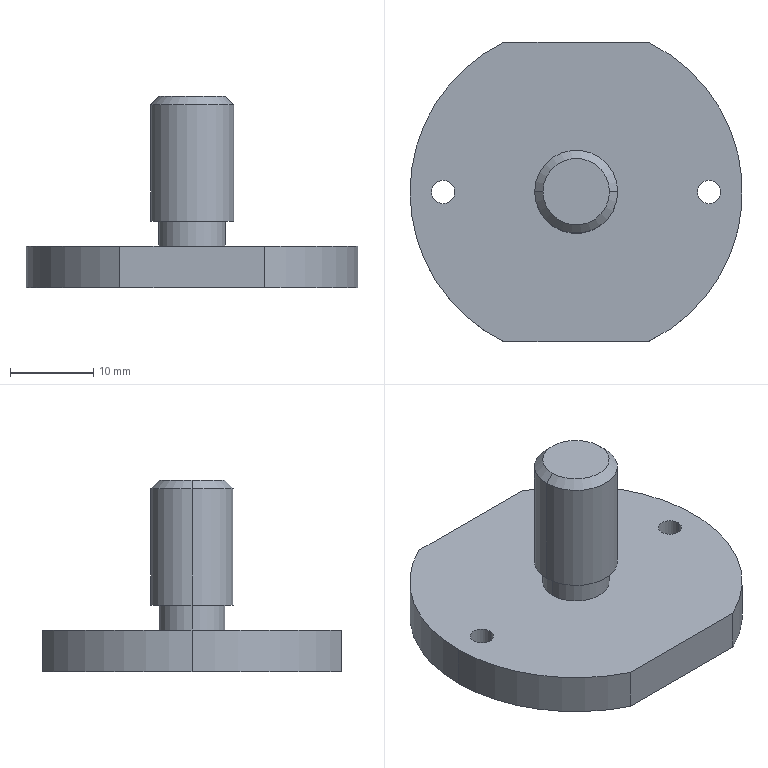Part | STEP file | Motor pulley screw | 1 solid | 19 faces | box 40 x 36 x 23 mm | volume 7301 mm3 | cylinder 11 | plane 6 | cone 2 | commonest cylinder face diameters 2.8 x4 40 x3 8 x2 10 x2
STEP:
#1=CARTESIAN_POINT('',(-14.6,0.,0.));
#2=VERTEX_POINT('',#1);
#3=CARTESIAN_POINT('',(-17.4,0.,0.));
#4=VERTEX_POINT('',#3);
#5=CARTESIAN_POINT('',(-16.,0.,0.));
#6=DIRECTION('',(0.,0.,-1.));
#7=DIRECTION('',(1.,0.,0.));
#8=AXIS2_PLACEMENT_3D('',#5,#6,#7);
#9=CIRCLE('',#8,1.4);
#10=EDGE_CURVE('',#2,#4,#9,.T.);
#11=ORIENTED_EDGE('',*,*,#10,.T.);
#12=CARTESIAN_POINT('',(-17.4,0.,5.));
#13=VERTEX_POINT('',#12);
#14=CARTESIAN_POINT('',(-17.4,0.,-10.));
#15=DIRECTION('',(0.,0.,1.));
#16=VECTOR('',#15,1000.);
#17=LINE('',#14,#16);
#18=EDGE_CURVE('',#4,#13,#17,.T.);
#19=ORIENTED_EDGE('',*,*,#18,.T.);
#20=CARTESIAN_POINT('',(-14.6,0.,5.));
#21=VERTEX_POINT('',#20);
#22=CARTESIAN_POINT('',(-16.,0.,5.));
#23=DIRECTION('',(0.,0.,-1.));
#24=DIRECTION('',(-1.,0.,0.));
#25=AXIS2_PLACEMENT_3D('',#22,#23,#24);
#26=CIRCLE('',#25,1.4);
#27=EDGE_CURVE('',#21,#13,#26,.T.);
#28=ORIENTED_EDGE('',*,*,#27,.F.);
#29=CARTESIAN_POINT('',(-14.6,0.,-10.));
#30=DIRECTION('',(0.,0.,1.));
#31=VECTOR('',#30,1000.);
#32=LINE('',#29,#31);
#33=EDGE_CURVE('',#2,#21,#32,.T.);
#34=ORIENTED_EDGE('',*,*,#33,.F.);
#35=EDGE_LOOP('',(#11,#19,#28,#34));
#36=FACE_OUTER_BOUND('',#35,.T.);
#37=CARTESIAN_POINT('',(-16.,0.,-10.));
#38=DIRECTION('',(0.,0.,1.));
#39=DIRECTION('',(1.,0.,0.));
#40=AXIS2_PLACEMENT_3D('',#37,#38,#39);
#41=CYLINDRICAL_SURFACE('',#40,1.4);
#42=ADVANCED_FACE('',(#36),#41,.F.);
#43=CARTESIAN_POINT('',(14.6,0.,0.));
#44=VERTEX_POINT('',#43);
#45=CARTESIAN_POINT('',(17.4,0.,0.));
#46=VERTEX_POINT('',#45);
#47=CARTESIAN_POINT('',(16.,0.,0.));
#48=DIRECTION('',(0.,0.,1.));
#49=DIRECTION('',(1.,0.,0.));
#50=AXIS2_PLACEMENT_3D('',#47,#48,#49);
#51=CIRCLE('',#50,1.4);
#52=EDGE_CURVE('',#44,#46,#51,.T.);
#53=ORIENTED_EDGE('',*,*,#52,.F.);
#54=CARTESIAN_POINT('',(14.6,0.,5.));
#55=VERTEX_POINT('',#54);
#56=CARTESIAN_POINT('',(14.6,0.,-10.));
#57=DIRECTION('',(0.,0.,1.));
#58=VECTOR('',#57,1000.);
#59=LINE('',#56,#58);
#60=EDGE_CURVE('',#44,#55,#59,.T.);
#61=ORIENTED_EDGE('',*,*,#60,.T.);
#62=CARTESIAN_POINT('',(17.4,0.,5.));
#63=VERTEX_POINT('',#62);
#64=CARTESIAN_POINT('',(16.,0.,5.));
#65=DIRECTION('',(0.,0.,1.));
#66=DIRECTION('',(1.,0.,0.));
#67=AXIS2_PLACEMENT_3D('',#64,#65,#66);
#68=CIRCLE('',#67,1.4);
#69=EDGE_CURVE('',#55,#63,#68,.T.);
#70=ORIENTED_EDGE('',*,*,#69,.T.);
#71=CARTESIAN_POINT('',(17.4,0.,-10.));
#72=DIRECTION('',(0.,0.,1.));
#73=VECTOR('',#72,1000.);
#74=LINE('',#71,#73);
#75=EDGE_CURVE('',#46,#63,#74,.T.);
#76=ORIENTED_EDGE('',*,*,#75,.F.);
#77=EDGE_LOOP('',(#53,#61,#70,#76));
#78=FACE_OUTER_BOUND('',#77,.T.);
#79=CARTESIAN_POINT('',(16.,0.,-10.));
#80=DIRECTION('',(0.,0.,1.));
#81=DIRECTION('',(1.,0.,0.));
#82=AXIS2_PLACEMENT_3D('',#79,#80,#81);
#83=CYLINDRICAL_SURFACE('',#82,1.4);
#84=ADVANCED_FACE('',(#78),#83,.F.);
#85=CARTESIAN_POINT('',(4.,0.,23.));
#86=VERTEX_POINT('',#85);
#87=CARTESIAN_POINT('',(-4.,0.,23.));
#88=VERTEX_POINT('',#87);
#89=CARTESIAN_POINT('',(0.,0.,23.));
#90=DIRECTION('',(0.,0.,1.));
#91=DIRECTION('',(1.,0.,0.));
#92=AXIS2_PLACEMENT_3D('',#89,#90,#91);
#93=CIRCLE('',#92,4.);
#94=EDGE_CURVE('',#86,#88,#93,.T.);
#95=ORIENTED_EDGE('',*,*,#94,.F.);
#96=CARTESIAN_POINT('',(5.,0.,22.));
#97=VERTEX_POINT('',#96);
#98=CARTESIAN_POINT('',(4.,0.,23.));
#99=DIRECTION('',(0.7071,0.,-0.7071));
#100=VECTOR('',#99,1000.);
#101=LINE('',#98,#100);
#102=EDGE_CURVE('',#86,#97,#101,.T.);
#103=ORIENTED_EDGE('',*,*,#102,.T.);
#104=CARTESIAN_POINT('',(-5.,0.,22.));
#105=VERTEX_POINT('',#104);
#106=CARTESIAN_POINT('',(0.,0.,22.));
#107=DIRECTION('',(0.,0.,-1.));
#108=DIRECTION('',(1.,0.,0.));
#109=AXIS2_PLACEMENT_3D('',#106,#107,#108);
#110=CIRCLE('',#109,5.);
#111=EDGE_CURVE('',#105,#97,#110,.T.);
#112=ORIENTED_EDGE('',*,*,#111,.F.);
#113=CARTESIAN_POINT('',(-4.,0.,23.));
#114=DIRECTION('',(-0.7071,0.,-0.7071));
#115=VECTOR('',#114,1000.);
#116=LINE('',#113,#115);
#117=EDGE_CURVE('',#88,#105,#116,.T.);
#118=ORIENTED_EDGE('',*,*,#117,.F.);
#119=EDGE_LOOP('',(#95,#103,#112,#118));
#120=FACE_OUTER_BOUND('',#119,.T.);
#121=CARTESIAN_POINT('',(0.,0.,23.));
#122=DIRECTION('',(0.,0.,-1.));
#123=DIRECTION('',(-1.,0.,0.));
#124=AXIS2_PLACEMENT_3D('',#121,#122,#123);
#125=CONICAL_SURFACE('',#124,4.,0.7854);
#126=ADVANCED_FACE('',(#120),#125,.T.);
#127=ORIENTED_EDGE('',*,*,#111,.T.);
#128=CARTESIAN_POINT('',(5.,0.,8.));
#129=VERTEX_POINT('',#128);
#130=CARTESIAN_POINT('',(5.,0.,23.));
#131=DIRECTION('',(0.,0.,-1.));
#132=VECTOR('',#131,1000.);
#133=LINE('',#130,#132);
#134=EDGE_CURVE('',#97,#129,#133,.T.);
#135=ORIENTED_EDGE('',*,*,#134,.T.);
#136=CARTESIAN_POINT('',(-5.,0.,8.));
#137=VERTEX_POINT('',#136);
#138=CARTESIAN_POINT('',(0.,0.,8.));
#139=DIRECTION('',(0.,0.,1.));
#140=DIRECTION('',(1.,0.,0.));
#141=AXIS2_PLACEMENT_3D('',#138,#139,#140);
#142=CIRCLE('',#141,5.);
#143=EDGE_CURVE('',#129,#137,#142,.T.);
#144=ORIENTED_EDGE('',*,*,#143,.T.);
#145=CARTESIAN_POINT('',(-5.,0.,23.));
#146=DIRECTION('',(0.,0.,-1.));
#147=VECTOR('',#146,1000.);
#148=LINE('',#145,#147);
#149=EDGE_CURVE('',#105,#137,#148,.T.);
#150=ORIENTED_EDGE('',*,*,#149,.F.);
#151=EDGE_LOOP('',(#127,#135,#144,#150));
#152=FACE_OUTER_BOUND('',#151,.T.);
#153=CARTESIAN_POINT('',(0.,0.,23.));
#154=DIRECTION('',(0.,0.,-1.));
#155=DIRECTION('',(-1.,0.,0.));
#156=AXIS2_PLACEMENT_3D('',#153,#154,#155);
#157=CYLINDRICAL_SURFACE('',#156,5.);
#158=ADVANCED_FACE('',(#152),#157,.T.);
#159=CARTESIAN_POINT('',(4.,0.,8.));
#160=VERTEX_POINT('',#159);
#161=CARTESIAN_POINT('',(-4.,0.,8.));
#162=VERTEX_POINT('',#161);
#163=CARTESIAN_POINT('',(0.,0.,8.));
#164=DIRECTION('',(0.,0.,1.));
#165=DIRECTION('',(1.,0.,0.));
#166=AXIS2_PLACEMENT_3D('',#163,#164,#165);
#167=CIRCLE('',#166,4.);
#168=EDGE_CURVE('',#160,#162,#167,.T.);
#169=ORIENTED_EDGE('',*,*,#168,.F.);
#170=CARTESIAN_POINT('',(4.,0.,5.));
#171=VERTEX_POINT('',#170);
#172=CARTESIAN_POINT('',(4.,0.,8.));
#173=DIRECTION('',(0.,0.,-1.));
#174=VECTOR('',#173,1000.);
#175=LINE('',#172,#174);
#176=EDGE_CURVE('',#160,#171,#175,.T.);
#177=ORIENTED_EDGE('',*,*,#176,.T.);
#178=CARTESIAN_POINT('',(-4.,0.,5.));
#179=VERTEX_POINT('',#178);
#180=CARTESIAN_POINT('',(0.,0.,5.));
#181=DIRECTION('',(0.,0.,1.));
#182=DIRECTION('',(1.,0.,0.));
#183=AXIS2_PLACEMENT_3D('',#180,#181,#182);
#184=CIRCLE('',#183,4.);
#185=EDGE_CURVE('',#171,#179,#184,.T.);
#186=ORIENTED_EDGE('',*,*,#185,.T.);
#187=CARTESIAN_POINT('',(-4.,0.,8.));
#188=DIRECTION('',(0.,0.,-1.));
#189=VECTOR('',#188,1000.);
#190=LINE('',#187,#189);
#191=EDGE_CURVE('',#162,#179,#190,.T.);
#192=ORIENTED_EDGE('',*,*,#191,.F.);
#193=EDGE_LOOP('',(#169,#177,#186,#192));
#194=FACE_OUTER_BOUND('',#193,.T.);
#195=CARTESIAN_POINT('',(0.,0.,8.));
#196=DIRECTION('',(0.,0.,-1.));
#197=DIRECTION('',(-1.,0.,0.));
#198=AXIS2_PLACEMENT_3D('',#195,#196,#197);
#199=CYLINDRICAL_SURFACE('',#198,4.);
#200=ADVANCED_FACE('',(#194),#199,.T.);
#201=CARTESIAN_POINT('',(-20.,0.,5.));
#202=VERTEX_POINT('',#201);
#203=CARTESIAN_POINT('',(-8.718,-18.,5.));
#204=VERTEX_POINT('',#203);
#205=CARTESIAN_POINT('',(0.,0.,5.));
#206=DIRECTION('',(0.,0.,1.));
#207=DIRECTION('',(1.,0.,0.));
#208=AXIS2_PLACEMENT_3D('',#205,#206,#207);
#209=CIRCLE('',#208,20.);
#210=EDGE_CURVE('',#202,#204,#209,.T.);
#211=ORIENTED_EDGE('',*,*,#210,.F.);
#212=CARTESIAN_POINT('',(-20.,0.,0.));
#213=VERTEX_POINT('',#212);
#214=CARTESIAN_POINT('',(-20.,0.,5.));
#215=DIRECTION('',(0.,0.,-1.));
#216=VECTOR('',#215,1000.);
#217=LINE('',#214,#216);
#218=EDGE_CURVE('',#202,#213,#217,.T.);
#219=ORIENTED_EDGE('',*,*,#218,.T.);
#220=CARTESIAN_POINT('',(-8.718,-18.,0.));
#221=VERTEX_POINT('',#220);
#222=CARTESIAN_POINT('',(0.,0.,0.));
#223=DIRECTION('',(0.,0.,1.));
#224=DIRECTION('',(1.,0.,0.));
#225=AXIS2_PLACEMENT_3D('',#222,#223,#224);
#226=CIRCLE('',#225,20.);
#227=EDGE_CURVE('',#213,#221,#226,.T.);
#228=ORIENTED_EDGE('',*,*,#227,.T.);
#229=CARTESIAN_POINT('',(-8.718,-18.,5.));
#230=DIRECTION('',(0.,0.,-1.));
#231=VECTOR('',#230,1000.);
#232=LINE('',#229,#231);
#233=EDGE_CURVE('',#204,#221,#232,.T.);
#234=ORIENTED_EDGE('',*,*,#233,.F.);
#235=EDGE_LOOP('',(#211,#219,#228,#234));
#236=FACE_OUTER_BOUND('',#235,.T.);
#237=CARTESIAN_POINT('',(0.,0.,5.));
#238=DIRECTION('',(0.,0.,-1.));
#239=DIRECTION('',(-1.,0.,0.));
#240=AXIS2_PLACEMENT_3D('',#237,#238,#239);
#241=CYLINDRICAL_SURFACE('',#240,20.);
#242=ADVANCED_FACE('',(#236),#241,.T.);
#243=ORIENTED_EDGE('',*,*,#218,.F.);
#244=CARTESIAN_POINT('',(-8.718,18.,5.));
#245=VERTEX_POINT('',#244);
#246=CARTESIAN_POINT('',(0.,0.,5.));
#247=DIRECTION('',(0.,0.,1.));
#248=DIRECTION('',(1.,0.,0.));
#249=AXIS2_PLACEMENT_3D('',#246,#247,#248);
#250=CIRCLE('',#249,20.);
#251=EDGE_CURVE('',#245,#202,#250,.T.);
#252=ORIENTED_EDGE('',*,*,#251,.F.);
#253=CARTESIAN_POINT('',(-8.718,18.,0.));
#254=VERTEX_POINT('',#253);
#255=CARTESIAN_POINT('',(-8.718,18.,5.));
#256=DIRECTION('',(0.,0.,-1.));
#257=VECTOR('',#256,1000.);
#258=LINE('',#255,#257);
#259=EDGE_CURVE('',#245,#254,#258,.T.);
#260=ORIENTED_EDGE('',*,*,#259,.T.);
#261=CARTESIAN_POINT('',(0.,0.,0.));
#262=DIRECTION('',(0.,0.,1.));
#263=DIRECTION('',(1.,0.,0.));
#264=AXIS2_PLACEMENT_3D('',#261,#262,#263);
#265=CIRCLE('',#264,20.);
#266=EDGE_CURVE('',#254,#213,#265,.T.);
#267=ORIENTED_EDGE('',*,*,#266,.T.);
#268=EDGE_LOOP('',(#243,#252,#260,#267));
#269=FACE_OUTER_BOUND('',#268,.T.);
#270=CARTESIAN_POINT('',(0.,0.,5.));
#271=DIRECTION('',(0.,0.,-1.));
#272=DIRECTION('',(-1.,0.,0.));
#273=AXIS2_PLACEMENT_3D('',#270,#271,#272);
#274=CYLINDRICAL_SURFACE('',#273,20.);
#275=ADVANCED_FACE('',(#269),#274,.T.);
#276=CARTESIAN_POINT('',(8.718,-18.,0.));
#277=VERTEX_POINT('',#276);
#278=CARTESIAN_POINT('',(8.718,-18.,5.));
#279=VERTEX_POINT('',#278);
#280=CARTESIAN_POINT('',(8.718,-18.,5.));
#281=DIRECTION('',(0.,0.,1.));
#282=VECTOR('',#281,1000.);
#283=LINE('',#280,#282);
#284=EDGE_CURVE('',#277,#279,#283,.T.);
#285=ORIENTED_EDGE('',*,*,#284,.F.);
#286=CARTESIAN_POINT('',(8.718,18.,0.));
#287=VERTEX_POINT('',#286);
#288=CARTESIAN_POINT('',(0.,0.,0.));
#289=DIRECTION('',(0.,0.,1.));
#290=DIRECTION('',(1.,0.,0.));
#291=AXIS2_PLACEMENT_3D('',#288,#289,#290);
#292=CIRCLE('',#291,20.);
#293=EDGE_CURVE('',#277,#287,#292,.T.);
#294=ORIENTED_EDGE('',*,*,#293,.T.);
#295=CARTESIAN_POINT('',(8.718,18.,5.));
#296=VERTEX_POINT('',#295);
#297=CARTESIAN_POINT('',(8.718,18.,5.));
#298=DIRECTION('',(0.,0.,1.));
#299=VECTOR('',#298,1000.);
#300=LINE('',#297,#299);
#301=EDGE_CURVE('',#287,#296,#300,.T.);
#302=ORIENTED_EDGE('',*,*,#301,.T.);
#303=CARTESIAN_POINT('',(0.,0.,5.));
#304=DIRECTION('',(0.,0.,1.));
#305=DIRECTION('',(1.,0.,0.));
#306=AXIS2_PLACEMENT_3D('',#303,#304,#305);
#307=CIRCLE('',#306,20.);
#308=EDGE_CURVE('',#279,#296,#307,.T.);
#309=ORIENTED_EDGE('',*,*,#308,.F.);
#310=EDGE_LOOP('',(#285,#294,#302,#309));
#311=FACE_OUTER_BOUND('',#310,.T.);
#312=CARTESIAN_POINT('',(0.,0.,5.));
#313=DIRECTION('',(0.,0.,-1.));
#314=DIRECTION('',(-1.,0.,0.));
#315=AXIS2_PLACEMENT_3D('',#312,#313,#314);
#316=CYLINDRICAL_SURFACE('',#315,20.);
#317=ADVANCED_FACE('',(#311),#316,.T.);
#318=ORIENTED_EDGE('',*,*,#27,.T.);
#319=CARTESIAN_POINT('',(-16.,0.,5.));
#320=DIRECTION('',(0.,0.,-1.));
#321=DIRECTION('',(-1.,0.,0.));
#322=AXIS2_PLACEMENT_3D('',#319,#320,#321);
#323=CIRCLE('',#322,1.4);
#324=EDGE_CURVE('',#13,#21,#323,.T.);
#325=ORIENTED_EDGE('',*,*,#324,.T.);
#326=EDGE_LOOP('',(#318,#325));
#327=FACE_BOUND('',#326,.T.);
#328=CARTESIAN_POINT('',(16.,0.,5.));
#329=DIRECTION('',(0.,0.,1.));
#330=DIRECTION('',(1.,0.,0.));
#331=AXIS2_PLACEMENT_3D('',#328,#329,#330);
#332=CIRCLE('',#331,1.4);
#333=EDGE_CURVE('',#63,#55,#332,.T.);
#334=ORIENTED_EDGE('',*,*,#333,.F.);
#335=ORIENTED_EDGE('',*,*,#69,.F.);
#336=EDGE_LOOP('',(#334,#335));
#337=FACE_BOUND('',#336,.T.);
#338=CARTESIAN_POINT('',(0.,0.,5.));
#339=DIRECTION('',(0.,0.,1.));
#340=DIRECTION('',(1.,0.,0.));
#341=AXIS2_PLACEMENT_3D('',#338,#339,#340);
#342=CIRCLE('',#341,4.);
#343=EDGE_CURVE('',#179,#171,#342,.T.);
#344=ORIENTED_EDGE('',*,*,#343,.F.);
#345=ORIENTED_EDGE('',*,*,#185,.F.);
#346=EDGE_LOOP('',(#344,#345));
#347=FACE_BOUND('',#346,.T.);
#348=ORIENTED_EDGE('',*,*,#251,.T.);
#349=ORIENTED_EDGE('',*,*,#210,.T.);
#350=CARTESIAN_POINT('',(11.985,-18.,5.));
#351=DIRECTION('',(1.,0.,0.));
#352=VECTOR('',#351,1000.);
#353=LINE('',#350,#352);
#354=EDGE_CURVE('',#204,#279,#353,.T.);
#355=ORIENTED_EDGE('',*,*,#354,.T.);
#356=ORIENTED_EDGE('',*,*,#308,.T.);
#357=CARTESIAN_POINT('',(11.985,18.,5.));
#358=DIRECTION('',(1.,0.,0.));
#359=VECTOR('',#358,1000.);
#360=LINE('',#357,#359);
#361=EDGE_CURVE('',#245,#296,#360,.T.);
#362=ORIENTED_EDGE('',*,*,#361,.F.);
#363=EDGE_LOOP('',(#348,#349,#355,#356,#362));
#364=FACE_OUTER_BOUND('',#363,.T.);
#365=CARTESIAN_POINT('',(0.,0.,5.));
#366=DIRECTION('',(0.,0.,1.));
#367=DIRECTION('',(1.,0.,0.));
#368=AXIS2_PLACEMENT_3D('',#365,#366,#367);
#369=PLANE('',#368);
#370=ADVANCED_FACE('',(#327,#337,#347,#364),#369,.T.);
#371=ORIENTED_EDGE('',*,*,#10,.F.);
#372=CARTESIAN_POINT('',(-16.,0.,0.));
#373=DIRECTION('',(0.,0.,-1.));
#374=DIRECTION('',(1.,0.,0.));
#375=AXIS2_PLACEMENT_3D('',#372,#373,#374);
#376=CIRCLE('',#375,1.4);
#377=EDGE_CURVE('',#4,#2,#376,.T.);
#378=ORIENTED_EDGE('',*,*,#377,.F.);
#379=EDGE_LOOP('',(#371,#378));
#380=FACE_BOUND('',#379,.T.);
#381=CARTESIAN_POINT('',(16.,0.,0.));
#382=DIRECTION('',(0.,0.,1.));
#383=DIRECTION('',(1.,0.,0.));
#384=AXIS2_PLACEMENT_3D('',#381,#382,#383);
#385=CIRCLE('',#384,1.4);
#386=EDGE_CURVE('',#46,#44,#385,.T.);
#387=ORIENTED_EDGE('',*,*,#386,.T.);
#388=ORIENTED_EDGE('',*,*,#52,.T.);
#389=EDGE_LOOP('',(#387,#388));
#390=FACE_BOUND('',#389,.T.);
#391=CARTESIAN_POINT('',(0.,-18.,0.));
#392=DIRECTION('',(1.,0.,0.));
#393=VECTOR('',#392,1000.);
#394=LINE('',#391,#393);
#395=EDGE_CURVE('',#221,#277,#394,.T.);
#396=ORIENTED_EDGE('',*,*,#395,.F.);
#397=ORIENTED_EDGE('',*,*,#227,.F.);
#398=ORIENTED_EDGE('',*,*,#266,.F.);
#399=CARTESIAN_POINT('',(0.,18.,0.));
#400=DIRECTION('',(1.,0.,0.));
#401=VECTOR('',#400,1000.);
#402=LINE('',#399,#401);
#403=EDGE_CURVE('',#254,#287,#402,.T.);
#404=ORIENTED_EDGE('',*,*,#403,.T.);
#405=ORIENTED_EDGE('',*,*,#293,.F.);
#406=EDGE_LOOP('',(#396,#397,#398,#404,#405));
#407=FACE_OUTER_BOUND('',#406,.T.);
#408=CARTESIAN_POINT('',(0.,0.,0.));
#409=DIRECTION('',(0.,0.,1.));
#410=DIRECTION('',(1.,0.,0.));
#411=AXIS2_PLACEMENT_3D('',#408,#409,#410);
#412=PLANE('',#411);
#413=ADVANCED_FACE('',(#380,#390,#407),#412,.F.);
#414=ORIENTED_EDGE('',*,*,#176,.F.);
#415=CARTESIAN_POINT('',(0.,0.,8.));
#416=DIRECTION('',(0.,0.,1.));
#417=DIRECTION('',(1.,0.,0.));
#418=AXIS2_PLACEMENT_3D('',#415,#416,#417);
#419=CIRCLE('',#418,4.);
#420=EDGE_CURVE('',#162,#160,#419,.T.);
#421=ORIENTED_EDGE('',*,*,#420,.F.);
#422=ORIENTED_EDGE('',*,*,#191,.T.);
#423=ORIENTED_EDGE('',*,*,#343,.T.);
#424=EDGE_LOOP('',(#414,#421,#422,#423));
#425=FACE_OUTER_BOUND('',#424,.T.);
#426=CARTESIAN_POINT('',(0.,0.,8.));
#427=DIRECTION('',(0.,0.,-1.));
#428=DIRECTION('',(-1.,0.,0.));
#429=AXIS2_PLACEMENT_3D('',#426,#427,#428);
#430=CYLINDRICAL_SURFACE('',#429,4.);
#431=ADVANCED_FACE('',(#425),#430,.T.);
#432=ORIENTED_EDGE('',*,*,#134,.F.);
#433=CARTESIAN_POINT('',(0.,0.,22.));
#434=DIRECTION('',(0.,0.,-1.));
#435=DIRECTION('',(1.,0.,0.));
#436=AXIS2_PLACEMENT_3D('',#433,#434,#435);
#437=CIRCLE('',#436,5.);
#438=EDGE_CURVE('',#97,#105,#437,.T.);
#439=ORIENTED_EDGE('',*,*,#438,.T.);
#440=ORIENTED_EDGE('',*,*,#149,.T.);
#441=CARTESIAN_POINT('',(0.,0.,8.));
#442=DIRECTION('',(0.,0.,1.));
#443=DIRECTION('',(1.,0.,0.));
#444=AXIS2_PLACEMENT_3D('',#441,#442,#443);
#445=CIRCLE('',#444,5.);
#446=EDGE_CURVE('',#137,#129,#445,.T.);
#447=ORIENTED_EDGE('',*,*,#446,.T.);
#448=EDGE_LOOP('',(#432,#439,#440,#447));
#449=FACE_OUTER_BOUND('',#448,.T.);
#450=CARTESIAN_POINT('',(0.,0.,23.));
#451=DIRECTION('',(0.,0.,-1.));
#452=DIRECTION('',(-1.,0.,0.));
#453=AXIS2_PLACEMENT_3D('',#450,#451,#452);
#454=CYLINDRICAL_SURFACE('',#453,5.);
#455=ADVANCED_FACE('',(#449),#454,.T.);
#456=CARTESIAN_POINT('',(0.,0.,23.));
#457=DIRECTION('',(0.,0.,1.));
#458=DIRECTION('',(1.,0.,0.));
#459=AXIS2_PLACEMENT_3D('',#456,#457,#458);
#460=CIRCLE('',#459,4.);
#461=EDGE_CURVE('',#88,#86,#460,.T.);
#462=ORIENTED_EDGE('',*,*,#461,.T.);
#463=ORIENTED_EDGE('',*,*,#94,.T.);
#464=EDGE_LOOP('',(#462,#463));
#465=FACE_OUTER_BOUND('',#464,.T.);
#466=CARTESIAN_POINT('',(0.,0.,23.));
#467=DIRECTION('',(0.,0.,1.));
#468=DIRECTION('',(1.,0.,0.));
#469=AXIS2_PLACEMENT_3D('',#466,#467,#468);
#470=PLANE('',#469);
#471=ADVANCED_FACE('',(#465),#470,.T.);
#472=ORIENTED_EDGE('',*,*,#420,.T.);
#473=ORIENTED_EDGE('',*,*,#168,.T.);
#474=EDGE_LOOP('',(#472,#473));
#475=FACE_BOUND('',#474,.T.);
#476=ORIENTED_EDGE('',*,*,#446,.F.);
#477=ORIENTED_EDGE('',*,*,#143,.F.);
#478=EDGE_LOOP('',(#476,#477));
#479=FACE_OUTER_BOUND('',#478,.T.);
#480=CARTESIAN_POINT('',(0.,0.,8.));
#481=DIRECTION('',(0.,0.,1.));
#482=DIRECTION('',(1.,0.,0.));
#483=AXIS2_PLACEMENT_3D('',#480,#481,#482);
#484=PLANE('',#483);
#485=ADVANCED_FACE('',(#475,#479),#484,.F.);
#486=ORIENTED_EDGE('',*,*,#102,.F.);
#487=ORIENTED_EDGE('',*,*,#461,.F.);
#488=ORIENTED_EDGE('',*,*,#117,.T.);
#489=ORIENTED_EDGE('',*,*,#438,.F.);
#490=EDGE_LOOP('',(#486,#487,#488,#489));
#491=FACE_OUTER_BOUND('',#490,.T.);
#492=CARTESIAN_POINT('',(0.,0.,23.));
#493=DIRECTION('',(0.,0.,-1.));
#494=DIRECTION('',(-1.,0.,0.));
#495=AXIS2_PLACEMENT_3D('',#492,#493,#494);
#496=CONICAL_SURFACE('',#495,4.,0.7854);
#497=ADVANCED_FACE('',(#491),#496,.T.);
#498=ORIENTED_EDGE('',*,*,#361,.T.);
#499=ORIENTED_EDGE('',*,*,#301,.F.);
#500=ORIENTED_EDGE('',*,*,#403,.F.);
#501=ORIENTED_EDGE('',*,*,#259,.F.);
#502=EDGE_LOOP('',(#498,#499,#500,#501));
#503=FACE_OUTER_BOUND('',#502,.T.);
#504=CARTESIAN_POINT('',(11.985,18.,-10.));
#505=DIRECTION('',(0.,-1.,0.));
#506=DIRECTION('',(0.,0.,-1.));
#507=AXIS2_PLACEMENT_3D('',#504,#505,#506);
#508=PLANE('',#507);
#509=ADVANCED_FACE('',(#503),#508,.F.);
#510=ORIENTED_EDGE('',*,*,#233,.T.);
#511=ORIENTED_EDGE('',*,*,#395,.T.);
#512=ORIENTED_EDGE('',*,*,#284,.T.);
#513=ORIENTED_EDGE('',*,*,#354,.F.);
#514=EDGE_LOOP('',(#510,#511,#512,#513));
#515=FACE_OUTER_BOUND('',#514,.T.);
#516=CARTESIAN_POINT('',(11.985,-18.,-10.));
#517=DIRECTION('',(0.,-1.,0.));
#518=DIRECTION('',(0.,0.,-1.));
#519=AXIS2_PLACEMENT_3D('',#516,#517,#518);
#520=PLANE('',#519);
#521=ADVANCED_FACE('',(#515),#520,.T.);
#522=ORIENTED_EDGE('',*,*,#60,.F.);
#523=ORIENTED_EDGE('',*,*,#386,.F.);
#524=ORIENTED_EDGE('',*,*,#75,.T.);
#525=ORIENTED_EDGE('',*,*,#333,.T.);
#526=EDGE_LOOP('',(#522,#523,#524,#525));
#527=FACE_OUTER_BOUND('',#526,.T.);
#528=CARTESIAN_POINT('',(16.,0.,-10.));
#529=DIRECTION('',(0.,0.,1.));
#530=DIRECTION('',(1.,0.,0.));
#531=AXIS2_PLACEMENT_3D('',#528,#529,#530);
#532=CYLINDRICAL_SURFACE('',#531,1.4);
#533=ADVANCED_FACE('',(#527),#532,.F.);
#534=ORIENTED_EDGE('',*,*,#18,.F.);
#535=ORIENTED_EDGE('',*,*,#377,.T.);
#536=ORIENTED_EDGE('',*,*,#33,.T.);
#537=ORIENTED_EDGE('',*,*,#324,.F.);
#538=EDGE_LOOP('',(#534,#535,#536,#537));
#539=FACE_OUTER_BOUND('',#538,.T.);
#540=CARTESIAN_POINT('',(-16.,0.,-10.));
#541=DIRECTION('',(0.,0.,1.));
#542=DIRECTION('',(1.,0.,0.));
#543=AXIS2_PLACEMENT_3D('',#540,#541,#542);
#544=CYLINDRICAL_SURFACE('',#543,1.4);
#545=ADVANCED_FACE('',(#539),#544,.F.);
#546=CLOSED_SHELL('',(#42,#84,#126,#158,#200,#242,#275,#317,#370,#413,#431,#455,#471,#485,#497,#509,#521,#533,#545));
#547=MANIFOLD_SOLID_BREP('',#546);
#548=CARTESIAN_POINT('',(0.,0.,0.));
#549=DIRECTION('',(0.,0.,1.));
#550=DIRECTION('',(1.,0.,0.));
#551=AXIS2_PLACEMENT_3D('',#548,#549,#550);
#552=(LENGTH_UNIT()NAMED_UNIT(*)SI_UNIT(.MILLI.,.METRE.));
#553=UNCERTAINTY_MEASURE_WITH_UNIT(LENGTH_MEASURE(0.00001),#552,'','');
#554=(NAMED_UNIT(*)PLANE_ANGLE_UNIT()SI_UNIT($,.RADIAN.));
#555=(NAMED_UNIT(*)SI_UNIT($,.STERADIAN.)SOLID_ANGLE_UNIT());
#556=(GEOMETRIC_REPRESENTATION_CONTEXT(3)GLOBAL_UNCERTAINTY_ASSIGNED_CONTEXT((#553))GLOBAL_UNIT_ASSIGNED_CONTEXT((#552,#554,#555))REPRESENTATION_CONTEXT('',''));
#557=ADVANCED_BREP_SHAPE_REPRESENTATION('',(#547,#551),#556);